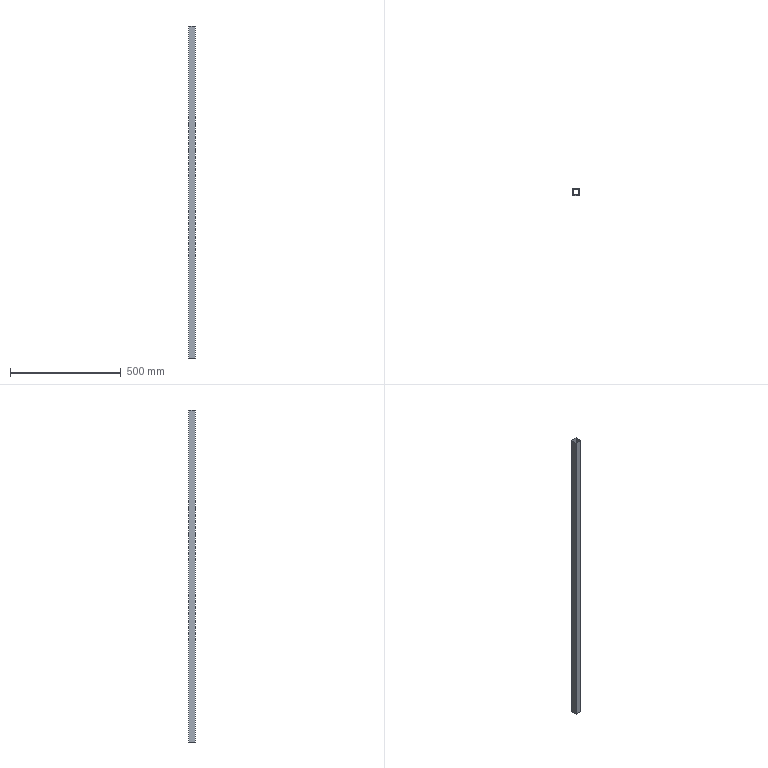Part | SolidWorks | features Extrusion 1 | 1 solid | 10 faces | box 30 x 30 x 1500 mm | volume 336000 mm3 | plane 10
STEP:
#1=CARTESIAN_POINT('',(-15.,15.,750.));
#2=VERTEX_POINT('',#1);
#3=CARTESIAN_POINT('',(-15.,-15.,750.));
#4=VERTEX_POINT('',#3);
#5=CARTESIAN_POINT('',(-15.,-15.,750.));
#6=DIRECTION('',(0.,-1.,0.));
#7=VECTOR('',#6,1000.);
#8=LINE('',#5,#7);
#9=EDGE_CURVE('',#2,#4,#8,.T.);
#10=ORIENTED_EDGE('',*,*,#9,.T.);
#11=CARTESIAN_POINT('',(15.,-15.,750.));
#12=VERTEX_POINT('',#11);
#13=CARTESIAN_POINT('',(15.,-15.,750.));
#14=DIRECTION('',(1.,0.,0.));
#15=VECTOR('',#14,1000.);
#16=LINE('',#13,#15);
#17=EDGE_CURVE('',#4,#12,#16,.T.);
#18=ORIENTED_EDGE('',*,*,#17,.T.);
#19=CARTESIAN_POINT('',(15.,15.,750.));
#20=VERTEX_POINT('',#19);
#21=CARTESIAN_POINT('',(15.,-15.,750.));
#22=DIRECTION('',(0.,1.,0.));
#23=VECTOR('',#22,1000.);
#24=LINE('',#21,#23);
#25=EDGE_CURVE('',#12,#20,#24,.T.);
#26=ORIENTED_EDGE('',*,*,#25,.T.);
#27=CARTESIAN_POINT('',(15.,15.,750.));
#28=DIRECTION('',(-1.,0.,0.));
#29=VECTOR('',#28,1000.);
#30=LINE('',#27,#29);
#31=EDGE_CURVE('',#20,#2,#30,.T.);
#32=ORIENTED_EDGE('',*,*,#31,.T.);
#33=EDGE_LOOP('',(#10,#18,#26,#32));
#34=FACE_OUTER_BOUND('',#33,.T.);
#35=CARTESIAN_POINT('',(13.,13.,750.));
#36=VERTEX_POINT('',#35);
#37=CARTESIAN_POINT('',(-13.,13.,750.));
#38=VERTEX_POINT('',#37);
#39=CARTESIAN_POINT('',(13.,13.,750.));
#40=DIRECTION('',(-1.,0.,0.));
#41=VECTOR('',#40,1000.);
#42=LINE('',#39,#41);
#43=EDGE_CURVE('',#36,#38,#42,.T.);
#44=ORIENTED_EDGE('',*,*,#43,.F.);
#45=CARTESIAN_POINT('',(13.,-13.,750.));
#46=VERTEX_POINT('',#45);
#47=CARTESIAN_POINT('',(13.,-13.,750.));
#48=DIRECTION('',(0.,1.,0.));
#49=VECTOR('',#48,1000.);
#50=LINE('',#47,#49);
#51=EDGE_CURVE('',#46,#36,#50,.T.);
#52=ORIENTED_EDGE('',*,*,#51,.F.);
#53=CARTESIAN_POINT('',(-13.,-13.,750.));
#54=VERTEX_POINT('',#53);
#55=CARTESIAN_POINT('',(13.,-13.,750.));
#56=DIRECTION('',(1.,0.,0.));
#57=VECTOR('',#56,1000.);
#58=LINE('',#55,#57);
#59=EDGE_CURVE('',#54,#46,#58,.T.);
#60=ORIENTED_EDGE('',*,*,#59,.F.);
#61=CARTESIAN_POINT('',(-13.,-13.,750.));
#62=DIRECTION('',(0.,-1.,0.));
#63=VECTOR('',#62,1000.);
#64=LINE('',#61,#63);
#65=EDGE_CURVE('',#38,#54,#64,.T.);
#66=ORIENTED_EDGE('',*,*,#65,.F.);
#67=EDGE_LOOP('',(#44,#52,#60,#66));
#68=FACE_BOUND('',#67,.T.);
#69=CARTESIAN_POINT('',(0.,0.,750.));
#70=DIRECTION('',(0.,0.,1.));
#71=DIRECTION('',(1.,0.,0.));
#72=AXIS2_PLACEMENT_3D('',#69,#70,#71);
#73=PLANE('',#72);
#74=ADVANCED_FACE('',(#34,#68),#73,.T.);
#75=CARTESIAN_POINT('',(-15.,15.,-750.));
#76=VERTEX_POINT('',#75);
#77=CARTESIAN_POINT('',(-15.,-15.,-750.));
#78=VERTEX_POINT('',#77);
#79=CARTESIAN_POINT('',(-15.,-15.,-750.));
#80=DIRECTION('',(0.,-1.,0.));
#81=VECTOR('',#80,1000.);
#82=LINE('',#79,#81);
#83=EDGE_CURVE('',#76,#78,#82,.T.);
#84=ORIENTED_EDGE('',*,*,#83,.F.);
#85=CARTESIAN_POINT('',(15.,15.,-750.));
#86=VERTEX_POINT('',#85);
#87=CARTESIAN_POINT('',(15.,15.,-750.));
#88=DIRECTION('',(-1.,0.,0.));
#89=VECTOR('',#88,1000.);
#90=LINE('',#87,#89);
#91=EDGE_CURVE('',#86,#76,#90,.T.);
#92=ORIENTED_EDGE('',*,*,#91,.F.);
#93=CARTESIAN_POINT('',(15.,-15.,-750.));
#94=VERTEX_POINT('',#93);
#95=CARTESIAN_POINT('',(15.,-15.,-750.));
#96=DIRECTION('',(0.,1.,0.));
#97=VECTOR('',#96,1000.);
#98=LINE('',#95,#97);
#99=EDGE_CURVE('',#94,#86,#98,.T.);
#100=ORIENTED_EDGE('',*,*,#99,.F.);
#101=CARTESIAN_POINT('',(15.,-15.,-750.));
#102=DIRECTION('',(1.,0.,0.));
#103=VECTOR('',#102,1000.);
#104=LINE('',#101,#103);
#105=EDGE_CURVE('',#78,#94,#104,.T.);
#106=ORIENTED_EDGE('',*,*,#105,.F.);
#107=EDGE_LOOP('',(#84,#92,#100,#106));
#108=FACE_OUTER_BOUND('',#107,.T.);
#109=CARTESIAN_POINT('',(13.,-13.,-750.));
#110=VERTEX_POINT('',#109);
#111=CARTESIAN_POINT('',(13.,13.,-750.));
#112=VERTEX_POINT('',#111);
#113=CARTESIAN_POINT('',(13.,-13.,-750.));
#114=DIRECTION('',(0.,1.,0.));
#115=VECTOR('',#114,1000.);
#116=LINE('',#113,#115);
#117=EDGE_CURVE('',#110,#112,#116,.T.);
#118=ORIENTED_EDGE('',*,*,#117,.T.);
#119=CARTESIAN_POINT('',(-13.,13.,-750.));
#120=VERTEX_POINT('',#119);
#121=CARTESIAN_POINT('',(13.,13.,-750.));
#122=DIRECTION('',(-1.,0.,0.));
#123=VECTOR('',#122,1000.);
#124=LINE('',#121,#123);
#125=EDGE_CURVE('',#112,#120,#124,.T.);
#126=ORIENTED_EDGE('',*,*,#125,.T.);
#127=CARTESIAN_POINT('',(-13.,-13.,-750.));
#128=VERTEX_POINT('',#127);
#129=CARTESIAN_POINT('',(-13.,-13.,-750.));
#130=DIRECTION('',(0.,-1.,0.));
#131=VECTOR('',#130,1000.);
#132=LINE('',#129,#131);
#133=EDGE_CURVE('',#120,#128,#132,.T.);
#134=ORIENTED_EDGE('',*,*,#133,.T.);
#135=CARTESIAN_POINT('',(13.,-13.,-750.));
#136=DIRECTION('',(1.,0.,0.));
#137=VECTOR('',#136,1000.);
#138=LINE('',#135,#137);
#139=EDGE_CURVE('',#128,#110,#138,.T.);
#140=ORIENTED_EDGE('',*,*,#139,.T.);
#141=EDGE_LOOP('',(#118,#126,#134,#140));
#142=FACE_BOUND('',#141,.T.);
#143=CARTESIAN_POINT('',(0.,0.,-750.));
#144=DIRECTION('',(0.,0.,1.));
#145=DIRECTION('',(1.,0.,0.));
#146=AXIS2_PLACEMENT_3D('',#143,#144,#145);
#147=PLANE('',#146);
#148=ADVANCED_FACE('',(#108,#142),#147,.F.);
#149=ORIENTED_EDGE('',*,*,#83,.T.);
#150=CARTESIAN_POINT('',(-15.,-15.,750.));
#151=DIRECTION('',(0.,0.,-1.));
#152=VECTOR('',#151,1000.);
#153=LINE('',#150,#152);
#154=EDGE_CURVE('',#4,#78,#153,.T.);
#155=ORIENTED_EDGE('',*,*,#154,.F.);
#156=ORIENTED_EDGE('',*,*,#9,.F.);
#157=CARTESIAN_POINT('',(-15.,15.,750.));
#158=DIRECTION('',(0.,0.,-1.));
#159=VECTOR('',#158,1000.);
#160=LINE('',#157,#159);
#161=EDGE_CURVE('',#2,#76,#160,.T.);
#162=ORIENTED_EDGE('',*,*,#161,.T.);
#163=EDGE_LOOP('',(#149,#155,#156,#162));
#164=FACE_OUTER_BOUND('',#163,.T.);
#165=CARTESIAN_POINT('',(-15.,-15.,750.));
#166=DIRECTION('',(1.,0.,0.));
#167=DIRECTION('',(0.,1.,0.));
#168=AXIS2_PLACEMENT_3D('',#165,#166,#167);
#169=PLANE('',#168);
#170=ADVANCED_FACE('',(#164),#169,.F.);
#171=ORIENTED_EDGE('',*,*,#105,.T.);
#172=CARTESIAN_POINT('',(15.,-15.,750.));
#173=DIRECTION('',(0.,0.,-1.));
#174=VECTOR('',#173,1000.);
#175=LINE('',#172,#174);
#176=EDGE_CURVE('',#12,#94,#175,.T.);
#177=ORIENTED_EDGE('',*,*,#176,.F.);
#178=ORIENTED_EDGE('',*,*,#17,.F.);
#179=ORIENTED_EDGE('',*,*,#154,.T.);
#180=EDGE_LOOP('',(#171,#177,#178,#179));
#181=FACE_OUTER_BOUND('',#180,.T.);
#182=CARTESIAN_POINT('',(15.,-15.,750.));
#183=DIRECTION('',(0.,1.,0.));
#184=DIRECTION('',(-1.,0.,0.));
#185=AXIS2_PLACEMENT_3D('',#182,#183,#184);
#186=PLANE('',#185);
#187=ADVANCED_FACE('',(#181),#186,.F.);
#188=ORIENTED_EDGE('',*,*,#99,.T.);
#189=CARTESIAN_POINT('',(15.,15.,750.));
#190=DIRECTION('',(0.,0.,-1.));
#191=VECTOR('',#190,1000.);
#192=LINE('',#189,#191);
#193=EDGE_CURVE('',#20,#86,#192,.T.);
#194=ORIENTED_EDGE('',*,*,#193,.F.);
#195=ORIENTED_EDGE('',*,*,#25,.F.);
#196=ORIENTED_EDGE('',*,*,#176,.T.);
#197=EDGE_LOOP('',(#188,#194,#195,#196));
#198=FACE_OUTER_BOUND('',#197,.T.);
#199=CARTESIAN_POINT('',(15.,-15.,750.));
#200=DIRECTION('',(-1.,0.,0.));
#201=DIRECTION('',(0.,0.,1.));
#202=AXIS2_PLACEMENT_3D('',#199,#200,#201);
#203=PLANE('',#202);
#204=ADVANCED_FACE('',(#198),#203,.F.);
#205=ORIENTED_EDGE('',*,*,#91,.T.);
#206=ORIENTED_EDGE('',*,*,#161,.F.);
#207=ORIENTED_EDGE('',*,*,#31,.F.);
#208=ORIENTED_EDGE('',*,*,#193,.T.);
#209=EDGE_LOOP('',(#205,#206,#207,#208));
#210=FACE_OUTER_BOUND('',#209,.T.);
#211=CARTESIAN_POINT('',(15.,15.,750.));
#212=DIRECTION('',(0.,-1.,0.));
#213=DIRECTION('',(0.,0.,-1.));
#214=AXIS2_PLACEMENT_3D('',#211,#212,#213);
#215=PLANE('',#214);
#216=ADVANCED_FACE('',(#210),#215,.F.);
#217=ORIENTED_EDGE('',*,*,#117,.F.);
#218=CARTESIAN_POINT('',(13.,-13.,750.));
#219=DIRECTION('',(0.,0.,-1.));
#220=VECTOR('',#219,1000.);
#221=LINE('',#218,#220);
#222=EDGE_CURVE('',#46,#110,#221,.T.);
#223=ORIENTED_EDGE('',*,*,#222,.F.);
#224=ORIENTED_EDGE('',*,*,#51,.T.);
#225=CARTESIAN_POINT('',(13.,13.,750.));
#226=DIRECTION('',(0.,0.,-1.));
#227=VECTOR('',#226,1000.);
#228=LINE('',#225,#227);
#229=EDGE_CURVE('',#36,#112,#228,.T.);
#230=ORIENTED_EDGE('',*,*,#229,.T.);
#231=EDGE_LOOP('',(#217,#223,#224,#230));
#232=FACE_OUTER_BOUND('',#231,.T.);
#233=CARTESIAN_POINT('',(13.,-13.,750.));
#234=DIRECTION('',(-1.,0.,0.));
#235=DIRECTION('',(0.,0.,1.));
#236=AXIS2_PLACEMENT_3D('',#233,#234,#235);
#237=PLANE('',#236);
#238=ADVANCED_FACE('',(#232),#237,.T.);
#239=ORIENTED_EDGE('',*,*,#125,.F.);
#240=ORIENTED_EDGE('',*,*,#229,.F.);
#241=ORIENTED_EDGE('',*,*,#43,.T.);
#242=CARTESIAN_POINT('',(-13.,13.,750.));
#243=DIRECTION('',(0.,0.,-1.));
#244=VECTOR('',#243,1000.);
#245=LINE('',#242,#244);
#246=EDGE_CURVE('',#38,#120,#245,.T.);
#247=ORIENTED_EDGE('',*,*,#246,.T.);
#248=EDGE_LOOP('',(#239,#240,#241,#247));
#249=FACE_OUTER_BOUND('',#248,.T.);
#250=CARTESIAN_POINT('',(13.,13.,750.));
#251=DIRECTION('',(0.,-1.,0.));
#252=DIRECTION('',(1.,0.,0.));
#253=AXIS2_PLACEMENT_3D('',#250,#251,#252);
#254=PLANE('',#253);
#255=ADVANCED_FACE('',(#249),#254,.T.);
#256=ORIENTED_EDGE('',*,*,#133,.F.);
#257=ORIENTED_EDGE('',*,*,#246,.F.);
#258=ORIENTED_EDGE('',*,*,#65,.T.);
#259=CARTESIAN_POINT('',(-13.,-13.,750.));
#260=DIRECTION('',(0.,0.,-1.));
#261=VECTOR('',#260,1000.);
#262=LINE('',#259,#261);
#263=EDGE_CURVE('',#54,#128,#262,.T.);
#264=ORIENTED_EDGE('',*,*,#263,.T.);
#265=EDGE_LOOP('',(#256,#257,#258,#264));
#266=FACE_OUTER_BOUND('',#265,.T.);
#267=CARTESIAN_POINT('',(-13.,-13.,750.));
#268=DIRECTION('',(1.,0.,0.));
#269=DIRECTION('',(0.,1.,0.));
#270=AXIS2_PLACEMENT_3D('',#267,#268,#269);
#271=PLANE('',#270);
#272=ADVANCED_FACE('',(#266),#271,.T.);
#273=ORIENTED_EDGE('',*,*,#139,.F.);
#274=ORIENTED_EDGE('',*,*,#263,.F.);
#275=ORIENTED_EDGE('',*,*,#59,.T.);
#276=ORIENTED_EDGE('',*,*,#222,.T.);
#277=EDGE_LOOP('',(#273,#274,#275,#276));
#278=FACE_OUTER_BOUND('',#277,.T.);
#279=CARTESIAN_POINT('',(13.,-13.,750.));
#280=DIRECTION('',(0.,1.,0.));
#281=DIRECTION('',(-1.,0.,0.));
#282=AXIS2_PLACEMENT_3D('',#279,#280,#281);
#283=PLANE('',#282);
#284=ADVANCED_FACE('',(#278),#283,.T.);
#285=CLOSED_SHELL('',(#74,#148,#170,#187,#204,#216,#238,#255,#272,#284));
#286=MANIFOLD_SOLID_BREP('',#285);
#287=CARTESIAN_POINT('',(0.,0.,0.));
#288=DIRECTION('',(0.,0.,1.));
#289=DIRECTION('',(1.,0.,0.));
#290=AXIS2_PLACEMENT_3D('',#287,#288,#289);
#291=(LENGTH_UNIT()NAMED_UNIT(*)SI_UNIT(.MILLI.,.METRE.));
#292=UNCERTAINTY_MEASURE_WITH_UNIT(LENGTH_MEASURE(0.00001),#291,'','');
#293=(NAMED_UNIT(*)PLANE_ANGLE_UNIT()SI_UNIT($,.RADIAN.));
#294=(NAMED_UNIT(*)SI_UNIT($,.STERADIAN.)SOLID_ANGLE_UNIT());
#295=(GEOMETRIC_REPRESENTATION_CONTEXT(3)GLOBAL_UNCERTAINTY_ASSIGNED_CONTEXT((#292))GLOBAL_UNIT_ASSIGNED_CONTEXT((#291,#293,#294))REPRESENTATION_CONTEXT('',''));
#296=ADVANCED_BREP_SHAPE_REPRESENTATION('',(#286,#290),#295);